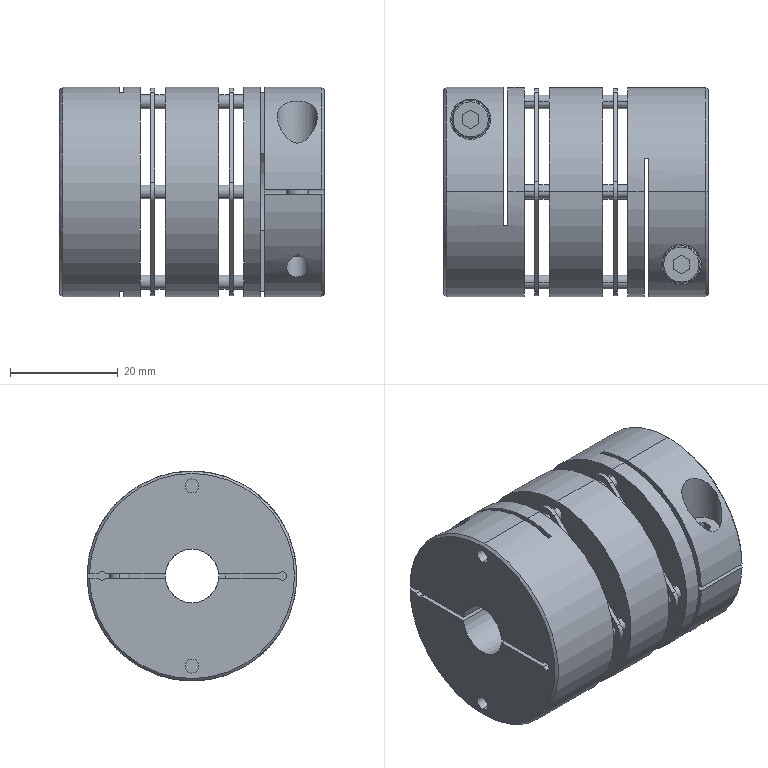Part | SolidWorks | features BaseBody 3 | 3 solids | 194 faces | box 49.2 x 39 x 39 mm | volume 37914 mm3 | cylinder 115 | plane 67 | cone 12 | commonest cylinder face diameters 2.6 x48 1.6 x12 4 x12 5.2 x10 39 x10 19.5 x6